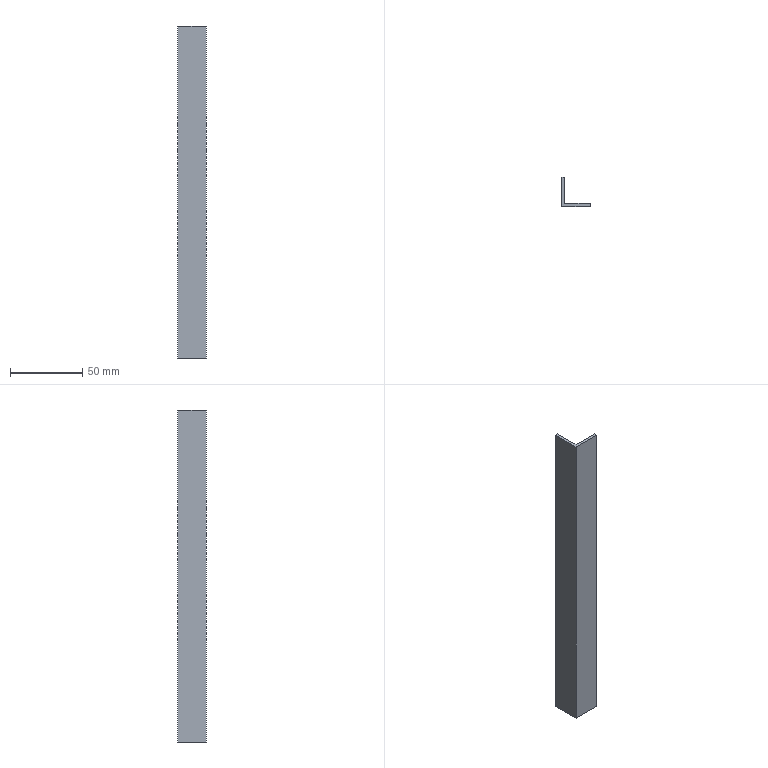Part | STEP file | BCC3 H16_15 | 1 solid | 8 faces | box 20 x 20 x 230 mm | volume 17480 mm3 | plane 8
STEP:
#1=CARTESIAN_POINT('',(0.,0.,0.));
#2=DIRECTION('',(0.,0.,1.));
#3=DIRECTION('',(1.,0.,0.));
#4=AXIS2_PLACEMENT_3D('',#1,#2,#3);
#5=CARTESIAN_POINT('',(0.,0.,-115.));
#6=VERTEX_POINT('',#5);
#7=CARTESIAN_POINT('',(20.,0.,-115.));
#8=VERTEX_POINT('',#7);
#9=CARTESIAN_POINT('',(0.,0.,-115.));
#10=DIRECTION('',(1.,0.,0.));
#11=VECTOR('',#10,1.);
#12=LINE('',#9,#11);
#13=CARTESIAN_POINT('',(0.,0.,115.));
#14=DIRECTION('',(0.,1.,0.));
#15=DIRECTION('',(0.,0.,1.));
#16=AXIS2_PLACEMENT_3D('',#13,#14,#15);
#17=PLANE('',#16);
#18=CARTESIAN_POINT('',(-230.,0.));
#19=DIRECTION('',(0.,1.));
#20=VECTOR('',#19,1.);
#21=LINE('',#18,#20);
#22=(GEOMETRIC_REPRESENTATION_CONTEXT(2)PARAMETRIC_REPRESENTATION_CONTEXT()REPRESENTATION_CONTEXT('',''));
#23=DEFINITIONAL_REPRESENTATION('',(#21),#22);
#24=PCURVE('',#17,#23);
#25=CARTESIAN_POINT('',(0.,0.,-115.));
#26=DIRECTION('',(0.,0.,1.));
#27=DIRECTION('',(1.,0.,0.));
#28=AXIS2_PLACEMENT_3D('',#25,#26,#27);
#29=PLANE('',#28);
#30=CARTESIAN_POINT('',(0.,0.));
#31=DIRECTION('',(1.,0.));
#32=VECTOR('',#31,1.);
#33=LINE('',#30,#32);
#34=(GEOMETRIC_REPRESENTATION_CONTEXT(2)PARAMETRIC_REPRESENTATION_CONTEXT()REPRESENTATION_CONTEXT('',''));
#35=DEFINITIONAL_REPRESENTATION('',(#33),#34);
#36=PCURVE('',#29,#35);
#37=SURFACE_CURVE('',#12,(#24,#36),.PCURVE_S1.);
#38=EDGE_CURVE('',#6,#8,#37,.T.);
#39=ORIENTED_EDGE('',*,*,#38,.T.);
#40=CARTESIAN_POINT('',(20.,0.,115.));
#41=VERTEX_POINT('',#40);
#42=CARTESIAN_POINT('',(20.,0.,115.));
#43=DIRECTION('',(0.,0.,-1.));
#44=VECTOR('',#43,1.);
#45=LINE('',#42,#44);
#46=CARTESIAN_POINT('',(0.,20.));
#47=DIRECTION('',(-1.,0.));
#48=VECTOR('',#47,1.);
#49=LINE('',#46,#48);
#50=(GEOMETRIC_REPRESENTATION_CONTEXT(2)PARAMETRIC_REPRESENTATION_CONTEXT()REPRESENTATION_CONTEXT('',''));
#51=DEFINITIONAL_REPRESENTATION('',(#49),#50);
#52=PCURVE('',#17,#51);
#53=CARTESIAN_POINT('',(20.,0.,115.));
#54=DIRECTION('',(-1.,0.,0.));
#55=DIRECTION('',(0.,0.,1.));
#56=AXIS2_PLACEMENT_3D('',#53,#54,#55);
#57=PLANE('',#56);
#58=CARTESIAN_POINT('',(0.,0.));
#59=DIRECTION('',(-1.,0.));
#60=VECTOR('',#59,1.);
#61=LINE('',#58,#60);
#62=(GEOMETRIC_REPRESENTATION_CONTEXT(2)PARAMETRIC_REPRESENTATION_CONTEXT()REPRESENTATION_CONTEXT('',''));
#63=DEFINITIONAL_REPRESENTATION('',(#61),#62);
#64=PCURVE('',#57,#63);
#65=SURFACE_CURVE('',#45,(#52,#64),.PCURVE_S1.);
#66=EDGE_CURVE('',#41,#8,#65,.T.);
#67=ORIENTED_EDGE('',*,*,#66,.F.);
#68=CARTESIAN_POINT('',(0.,0.,115.));
#69=VERTEX_POINT('',#68);
#70=CARTESIAN_POINT('',(0.,0.,115.));
#71=DIRECTION('',(1.,0.,0.));
#72=VECTOR('',#71,1.);
#73=LINE('',#70,#72);
#74=CARTESIAN_POINT('',(0.,0.));
#75=DIRECTION('',(0.,1.));
#76=VECTOR('',#75,1.);
#77=LINE('',#74,#76);
#78=(GEOMETRIC_REPRESENTATION_CONTEXT(2)PARAMETRIC_REPRESENTATION_CONTEXT()REPRESENTATION_CONTEXT('',''));
#79=DEFINITIONAL_REPRESENTATION('',(#77),#78);
#80=PCURVE('',#17,#79);
#81=CARTESIAN_POINT('',(0.,0.,115.));
#82=DIRECTION('',(0.,0.,1.));
#83=DIRECTION('',(1.,0.,0.));
#84=AXIS2_PLACEMENT_3D('',#81,#82,#83);
#85=PLANE('',#84);
#86=CARTESIAN_POINT('',(0.,0.));
#87=DIRECTION('',(1.,0.));
#88=VECTOR('',#87,1.);
#89=LINE('',#86,#88);
#90=(GEOMETRIC_REPRESENTATION_CONTEXT(2)PARAMETRIC_REPRESENTATION_CONTEXT()REPRESENTATION_CONTEXT('',''));
#91=DEFINITIONAL_REPRESENTATION('',(#89),#90);
#92=PCURVE('',#85,#91);
#93=SURFACE_CURVE('',#73,(#80,#92),.PCURVE_S1.);
#94=EDGE_CURVE('',#69,#41,#93,.T.);
#95=ORIENTED_EDGE('',*,*,#94,.F.);
#96=CARTESIAN_POINT('',(0.,0.,115.));
#97=DIRECTION('',(0.,0.,-1.));
#98=VECTOR('',#97,1.);
#99=LINE('',#96,#98);
#100=CARTESIAN_POINT('',(0.,0.));
#101=DIRECTION('',(-1.,0.));
#102=VECTOR('',#101,1.);
#103=LINE('',#100,#102);
#104=(GEOMETRIC_REPRESENTATION_CONTEXT(2)PARAMETRIC_REPRESENTATION_CONTEXT()REPRESENTATION_CONTEXT('',''));
#105=DEFINITIONAL_REPRESENTATION('',(#103),#104);
#106=PCURVE('',#17,#105);
#107=CARTESIAN_POINT('',(0.,0.,115.));
#108=DIRECTION('',(1.,0.,0.));
#109=DIRECTION('',(0.,0.,-1.));
#110=AXIS2_PLACEMENT_3D('',#107,#108,#109);
#111=PLANE('',#110);
#112=CARTESIAN_POINT('',(0.,0.));
#113=DIRECTION('',(1.,0.));
#114=VECTOR('',#113,1.);
#115=LINE('',#112,#114);
#116=(GEOMETRIC_REPRESENTATION_CONTEXT(2)PARAMETRIC_REPRESENTATION_CONTEXT()REPRESENTATION_CONTEXT('',''));
#117=DEFINITIONAL_REPRESENTATION('',(#115),#116);
#118=PCURVE('',#111,#117);
#119=SURFACE_CURVE('',#99,(#106,#118),.PCURVE_S1.);
#120=EDGE_CURVE('',#69,#6,#119,.T.);
#121=ORIENTED_EDGE('',*,*,#120,.T.);
#122=EDGE_LOOP('',(#39,#67,#95,#121));
#123=FACE_BOUND('',#122,.T.);
#124=ADVANCED_FACE('',(#123),#17,.F.);
#125=CARTESIAN_POINT('',(20.,2.,-115.));
#126=VERTEX_POINT('',#125);
#127=CARTESIAN_POINT('',(20.,0.,-115.));
#128=DIRECTION('',(0.,1.,0.));
#129=VECTOR('',#128,1.);
#130=LINE('',#127,#129);
#131=CARTESIAN_POINT('',(-230.,0.));
#132=DIRECTION('',(0.,1.));
#133=VECTOR('',#132,1.);
#134=LINE('',#131,#133);
#135=(GEOMETRIC_REPRESENTATION_CONTEXT(2)PARAMETRIC_REPRESENTATION_CONTEXT()REPRESENTATION_CONTEXT('',''));
#136=DEFINITIONAL_REPRESENTATION('',(#134),#135);
#137=PCURVE('',#57,#136);
#138=CARTESIAN_POINT('',(20.,0.));
#139=DIRECTION('',(0.,1.));
#140=VECTOR('',#139,1.);
#141=LINE('',#138,#140);
#142=(GEOMETRIC_REPRESENTATION_CONTEXT(2)PARAMETRIC_REPRESENTATION_CONTEXT()REPRESENTATION_CONTEXT('',''));
#143=DEFINITIONAL_REPRESENTATION('',(#141),#142);
#144=PCURVE('',#29,#143);
#145=SURFACE_CURVE('',#130,(#137,#144),.PCURVE_S1.);
#146=EDGE_CURVE('',#8,#126,#145,.T.);
#147=ORIENTED_EDGE('',*,*,#146,.T.);
#148=CARTESIAN_POINT('',(20.,2.,115.));
#149=VERTEX_POINT('',#148);
#150=CARTESIAN_POINT('',(20.,2.,115.));
#151=DIRECTION('',(0.,0.,-1.));
#152=VECTOR('',#151,1.);
#153=LINE('',#150,#152);
#154=CARTESIAN_POINT('',(0.,2.));
#155=DIRECTION('',(-1.,0.));
#156=VECTOR('',#155,1.);
#157=LINE('',#154,#156);
#158=(GEOMETRIC_REPRESENTATION_CONTEXT(2)PARAMETRIC_REPRESENTATION_CONTEXT()REPRESENTATION_CONTEXT('',''));
#159=DEFINITIONAL_REPRESENTATION('',(#157),#158);
#160=PCURVE('',#57,#159);
#161=CARTESIAN_POINT('',(20.,2.,115.));
#162=DIRECTION('',(0.,-1.,0.));
#163=DIRECTION('',(1.,0.,0.));
#164=AXIS2_PLACEMENT_3D('',#161,#162,#163);
#165=PLANE('',#164);
#166=CARTESIAN_POINT('',(0.,0.));
#167=DIRECTION('',(0.,-1.));
#168=VECTOR('',#167,1.);
#169=LINE('',#166,#168);
#170=(GEOMETRIC_REPRESENTATION_CONTEXT(2)PARAMETRIC_REPRESENTATION_CONTEXT()REPRESENTATION_CONTEXT('',''));
#171=DEFINITIONAL_REPRESENTATION('',(#169),#170);
#172=PCURVE('',#165,#171);
#173=SURFACE_CURVE('',#153,(#160,#172),.PCURVE_S1.);
#174=EDGE_CURVE('',#149,#126,#173,.T.);
#175=ORIENTED_EDGE('',*,*,#174,.F.);
#176=CARTESIAN_POINT('',(20.,0.,115.));
#177=DIRECTION('',(0.,1.,0.));
#178=VECTOR('',#177,1.);
#179=LINE('',#176,#178);
#180=CARTESIAN_POINT('',(0.,0.));
#181=DIRECTION('',(0.,1.));
#182=VECTOR('',#181,1.);
#183=LINE('',#180,#182);
#184=(GEOMETRIC_REPRESENTATION_CONTEXT(2)PARAMETRIC_REPRESENTATION_CONTEXT()REPRESENTATION_CONTEXT('',''));
#185=DEFINITIONAL_REPRESENTATION('',(#183),#184);
#186=PCURVE('',#57,#185);
#187=CARTESIAN_POINT('',(20.,0.));
#188=DIRECTION('',(0.,1.));
#189=VECTOR('',#188,1.);
#190=LINE('',#187,#189);
#191=(GEOMETRIC_REPRESENTATION_CONTEXT(2)PARAMETRIC_REPRESENTATION_CONTEXT()REPRESENTATION_CONTEXT('',''));
#192=DEFINITIONAL_REPRESENTATION('',(#190),#191);
#193=PCURVE('',#85,#192);
#194=SURFACE_CURVE('',#179,(#186,#193),.PCURVE_S1.);
#195=EDGE_CURVE('',#41,#149,#194,.T.);
#196=ORIENTED_EDGE('',*,*,#195,.F.);
#197=ORIENTED_EDGE('',*,*,#66,.T.);
#198=EDGE_LOOP('',(#147,#175,#196,#197));
#199=FACE_BOUND('',#198,.T.);
#200=ADVANCED_FACE('',(#199),#57,.F.);
#201=CARTESIAN_POINT('',(2.,2.,-115.));
#202=VERTEX_POINT('',#201);
#203=CARTESIAN_POINT('',(20.,2.,-115.));
#204=DIRECTION('',(-1.,0.,0.));
#205=VECTOR('',#204,1.);
#206=LINE('',#203,#205);
#207=CARTESIAN_POINT('',(0.,-230.));
#208=DIRECTION('',(-1.,0.));
#209=VECTOR('',#208,1.);
#210=LINE('',#207,#209);
#211=(GEOMETRIC_REPRESENTATION_CONTEXT(2)PARAMETRIC_REPRESENTATION_CONTEXT()REPRESENTATION_CONTEXT('',''));
#212=DEFINITIONAL_REPRESENTATION('',(#210),#211);
#213=PCURVE('',#165,#212);
#214=CARTESIAN_POINT('',(20.,2.));
#215=DIRECTION('',(-1.,0.));
#216=VECTOR('',#215,1.);
#217=LINE('',#214,#216);
#218=(GEOMETRIC_REPRESENTATION_CONTEXT(2)PARAMETRIC_REPRESENTATION_CONTEXT()REPRESENTATION_CONTEXT('',''));
#219=DEFINITIONAL_REPRESENTATION('',(#217),#218);
#220=PCURVE('',#29,#219);
#221=SURFACE_CURVE('',#206,(#213,#220),.PCURVE_S1.);
#222=EDGE_CURVE('',#126,#202,#221,.T.);
#223=ORIENTED_EDGE('',*,*,#222,.T.);
#224=CARTESIAN_POINT('',(2.,2.,115.));
#225=VERTEX_POINT('',#224);
#226=CARTESIAN_POINT('',(2.,2.,115.));
#227=DIRECTION('',(0.,0.,-1.));
#228=VECTOR('',#227,1.);
#229=LINE('',#226,#228);
#230=CARTESIAN_POINT('',(-18.,0.));
#231=DIRECTION('',(0.,-1.));
#232=VECTOR('',#231,1.);
#233=LINE('',#230,#232);
#234=(GEOMETRIC_REPRESENTATION_CONTEXT(2)PARAMETRIC_REPRESENTATION_CONTEXT()REPRESENTATION_CONTEXT('',''));
#235=DEFINITIONAL_REPRESENTATION('',(#233),#234);
#236=PCURVE('',#165,#235);
#237=CARTESIAN_POINT('',(2.,2.,115.));
#238=DIRECTION('',(-1.,0.,0.));
#239=DIRECTION('',(0.,-1.,0.));
#240=AXIS2_PLACEMENT_3D('',#237,#238,#239);
#241=PLANE('',#240);
#242=CARTESIAN_POINT('',(0.,0.));
#243=DIRECTION('',(0.,-1.));
#244=VECTOR('',#243,1.);
#245=LINE('',#242,#244);
#246=(GEOMETRIC_REPRESENTATION_CONTEXT(2)PARAMETRIC_REPRESENTATION_CONTEXT()REPRESENTATION_CONTEXT('',''));
#247=DEFINITIONAL_REPRESENTATION('',(#245),#246);
#248=PCURVE('',#241,#247);
#249=SURFACE_CURVE('',#229,(#236,#248),.PCURVE_S1.);
#250=EDGE_CURVE('',#225,#202,#249,.T.);
#251=ORIENTED_EDGE('',*,*,#250,.F.);
#252=CARTESIAN_POINT('',(20.,2.,115.));
#253=DIRECTION('',(-1.,0.,0.));
#254=VECTOR('',#253,1.);
#255=LINE('',#252,#254);
#256=CARTESIAN_POINT('',(0.,0.));
#257=DIRECTION('',(-1.,0.));
#258=VECTOR('',#257,1.);
#259=LINE('',#256,#258);
#260=(GEOMETRIC_REPRESENTATION_CONTEXT(2)PARAMETRIC_REPRESENTATION_CONTEXT()REPRESENTATION_CONTEXT('',''));
#261=DEFINITIONAL_REPRESENTATION('',(#259),#260);
#262=PCURVE('',#165,#261);
#263=CARTESIAN_POINT('',(20.,2.));
#264=DIRECTION('',(-1.,0.));
#265=VECTOR('',#264,1.);
#266=LINE('',#263,#265);
#267=(GEOMETRIC_REPRESENTATION_CONTEXT(2)PARAMETRIC_REPRESENTATION_CONTEXT()REPRESENTATION_CONTEXT('',''));
#268=DEFINITIONAL_REPRESENTATION('',(#266),#267);
#269=PCURVE('',#85,#268);
#270=SURFACE_CURVE('',#255,(#262,#269),.PCURVE_S1.);
#271=EDGE_CURVE('',#149,#225,#270,.T.);
#272=ORIENTED_EDGE('',*,*,#271,.F.);
#273=ORIENTED_EDGE('',*,*,#174,.T.);
#274=EDGE_LOOP('',(#223,#251,#272,#273));
#275=FACE_BOUND('',#274,.T.);
#276=ADVANCED_FACE('',(#275),#165,.F.);
#277=CARTESIAN_POINT('',(2.,20.,-115.));
#278=VERTEX_POINT('',#277);
#279=CARTESIAN_POINT('',(2.,2.,-115.));
#280=DIRECTION('',(0.,1.,0.));
#281=VECTOR('',#280,1.);
#282=LINE('',#279,#281);
#283=CARTESIAN_POINT('',(0.,-230.));
#284=DIRECTION('',(-1.,0.));
#285=VECTOR('',#284,1.);
#286=LINE('',#283,#285);
#287=(GEOMETRIC_REPRESENTATION_CONTEXT(2)PARAMETRIC_REPRESENTATION_CONTEXT()REPRESENTATION_CONTEXT('',''));
#288=DEFINITIONAL_REPRESENTATION('',(#286),#287);
#289=PCURVE('',#241,#288);
#290=CARTESIAN_POINT('',(2.,2.));
#291=DIRECTION('',(0.,1.));
#292=VECTOR('',#291,1.);
#293=LINE('',#290,#292);
#294=(GEOMETRIC_REPRESENTATION_CONTEXT(2)PARAMETRIC_REPRESENTATION_CONTEXT()REPRESENTATION_CONTEXT('',''));
#295=DEFINITIONAL_REPRESENTATION('',(#293),#294);
#296=PCURVE('',#29,#295);
#297=SURFACE_CURVE('',#282,(#289,#296),.PCURVE_S1.);
#298=EDGE_CURVE('',#202,#278,#297,.T.);
#299=ORIENTED_EDGE('',*,*,#298,.T.);
#300=CARTESIAN_POINT('',(2.,20.,115.));
#301=VERTEX_POINT('',#300);
#302=CARTESIAN_POINT('',(2.,20.,115.));
#303=DIRECTION('',(0.,0.,-1.));
#304=VECTOR('',#303,1.);
#305=LINE('',#302,#304);
#306=CARTESIAN_POINT('',(-18.,0.));
#307=DIRECTION('',(0.,-1.));
#308=VECTOR('',#307,1.);
#309=LINE('',#306,#308);
#310=(GEOMETRIC_REPRESENTATION_CONTEXT(2)PARAMETRIC_REPRESENTATION_CONTEXT()REPRESENTATION_CONTEXT('',''));
#311=DEFINITIONAL_REPRESENTATION('',(#309),#310);
#312=PCURVE('',#241,#311);
#313=CARTESIAN_POINT('',(2.,20.,115.));
#314=DIRECTION('',(0.,-1.,0.));
#315=DIRECTION('',(0.,0.,-1.));
#316=AXIS2_PLACEMENT_3D('',#313,#314,#315);
#317=PLANE('',#316);
#318=CARTESIAN_POINT('',(0.,0.));
#319=DIRECTION('',(1.,0.));
#320=VECTOR('',#319,1.);
#321=LINE('',#318,#320);
#322=(GEOMETRIC_REPRESENTATION_CONTEXT(2)PARAMETRIC_REPRESENTATION_CONTEXT()REPRESENTATION_CONTEXT('',''));
#323=DEFINITIONAL_REPRESENTATION('',(#321),#322);
#324=PCURVE('',#317,#323);
#325=SURFACE_CURVE('',#305,(#312,#324),.PCURVE_S1.);
#326=EDGE_CURVE('',#301,#278,#325,.T.);
#327=ORIENTED_EDGE('',*,*,#326,.F.);
#328=CARTESIAN_POINT('',(2.,2.,115.));
#329=DIRECTION('',(0.,1.,0.));
#330=VECTOR('',#329,1.);
#331=LINE('',#328,#330);
#332=CARTESIAN_POINT('',(0.,0.));
#333=DIRECTION('',(-1.,0.));
#334=VECTOR('',#333,1.);
#335=LINE('',#332,#334);
#336=(GEOMETRIC_REPRESENTATION_CONTEXT(2)PARAMETRIC_REPRESENTATION_CONTEXT()REPRESENTATION_CONTEXT('',''));
#337=DEFINITIONAL_REPRESENTATION('',(#335),#336);
#338=PCURVE('',#241,#337);
#339=CARTESIAN_POINT('',(2.,2.));
#340=DIRECTION('',(0.,1.));
#341=VECTOR('',#340,1.);
#342=LINE('',#339,#341);
#343=(GEOMETRIC_REPRESENTATION_CONTEXT(2)PARAMETRIC_REPRESENTATION_CONTEXT()REPRESENTATION_CONTEXT('',''));
#344=DEFINITIONAL_REPRESENTATION('',(#342),#343);
#345=PCURVE('',#85,#344);
#346=SURFACE_CURVE('',#331,(#338,#345),.PCURVE_S1.);
#347=EDGE_CURVE('',#225,#301,#346,.T.);
#348=ORIENTED_EDGE('',*,*,#347,.F.);
#349=ORIENTED_EDGE('',*,*,#250,.T.);
#350=EDGE_LOOP('',(#299,#327,#348,#349));
#351=FACE_BOUND('',#350,.T.);
#352=ADVANCED_FACE('',(#351),#241,.F.);
#353=CARTESIAN_POINT('',(0.,20.,-115.));
#354=VERTEX_POINT('',#353);
#355=CARTESIAN_POINT('',(2.,20.,-115.));
#356=DIRECTION('',(-1.,0.,0.));
#357=VECTOR('',#356,1.);
#358=LINE('',#355,#357);
#359=CARTESIAN_POINT('',(230.,0.));
#360=DIRECTION('',(0.,-1.));
#361=VECTOR('',#360,1.);
#362=LINE('',#359,#361);
#363=(GEOMETRIC_REPRESENTATION_CONTEXT(2)PARAMETRIC_REPRESENTATION_CONTEXT()REPRESENTATION_CONTEXT('',''));
#364=DEFINITIONAL_REPRESENTATION('',(#362),#363);
#365=PCURVE('',#317,#364);
#366=CARTESIAN_POINT('',(2.,20.));
#367=DIRECTION('',(-1.,0.));
#368=VECTOR('',#367,1.);
#369=LINE('',#366,#368);
#370=(GEOMETRIC_REPRESENTATION_CONTEXT(2)PARAMETRIC_REPRESENTATION_CONTEXT()REPRESENTATION_CONTEXT('',''));
#371=DEFINITIONAL_REPRESENTATION('',(#369),#370);
#372=PCURVE('',#29,#371);
#373=SURFACE_CURVE('',#358,(#365,#372),.PCURVE_S1.);
#374=EDGE_CURVE('',#278,#354,#373,.T.);
#375=ORIENTED_EDGE('',*,*,#374,.T.);
#376=CARTESIAN_POINT('',(0.,20.,115.));
#377=VERTEX_POINT('',#376);
#378=CARTESIAN_POINT('',(0.,20.,115.));
#379=DIRECTION('',(0.,0.,-1.));
#380=VECTOR('',#379,1.);
#381=LINE('',#378,#380);
#382=CARTESIAN_POINT('',(0.,-2.));
#383=DIRECTION('',(1.,0.));
#384=VECTOR('',#383,1.);
#385=LINE('',#382,#384);
#386=(GEOMETRIC_REPRESENTATION_CONTEXT(2)PARAMETRIC_REPRESENTATION_CONTEXT()REPRESENTATION_CONTEXT('',''));
#387=DEFINITIONAL_REPRESENTATION('',(#385),#386);
#388=PCURVE('',#317,#387);
#389=CARTESIAN_POINT('',(0.,20.));
#390=DIRECTION('',(1.,0.));
#391=VECTOR('',#390,1.);
#392=LINE('',#389,#391);
#393=(GEOMETRIC_REPRESENTATION_CONTEXT(2)PARAMETRIC_REPRESENTATION_CONTEXT()REPRESENTATION_CONTEXT('',''));
#394=DEFINITIONAL_REPRESENTATION('',(#392),#393);
#395=PCURVE('',#111,#394);
#396=SURFACE_CURVE('',#381,(#388,#395),.PCURVE_S1.);
#397=EDGE_CURVE('',#377,#354,#396,.T.);
#398=ORIENTED_EDGE('',*,*,#397,.F.);
#399=CARTESIAN_POINT('',(2.,20.,115.));
#400=DIRECTION('',(-1.,0.,0.));
#401=VECTOR('',#400,1.);
#402=LINE('',#399,#401);
#403=CARTESIAN_POINT('',(0.,0.));
#404=DIRECTION('',(0.,-1.));
#405=VECTOR('',#404,1.);
#406=LINE('',#403,#405);
#407=(GEOMETRIC_REPRESENTATION_CONTEXT(2)PARAMETRIC_REPRESENTATION_CONTEXT()REPRESENTATION_CONTEXT('',''));
#408=DEFINITIONAL_REPRESENTATION('',(#406),#407);
#409=PCURVE('',#317,#408);
#410=CARTESIAN_POINT('',(2.,20.));
#411=DIRECTION('',(-1.,0.));
#412=VECTOR('',#411,1.);
#413=LINE('',#410,#412);
#414=(GEOMETRIC_REPRESENTATION_CONTEXT(2)PARAMETRIC_REPRESENTATION_CONTEXT()REPRESENTATION_CONTEXT('',''));
#415=DEFINITIONAL_REPRESENTATION('',(#413),#414);
#416=PCURVE('',#85,#415);
#417=SURFACE_CURVE('',#402,(#409,#416),.PCURVE_S1.);
#418=EDGE_CURVE('',#301,#377,#417,.T.);
#419=ORIENTED_EDGE('',*,*,#418,.F.);
#420=ORIENTED_EDGE('',*,*,#326,.T.);
#421=EDGE_LOOP('',(#375,#398,#419,#420));
#422=FACE_BOUND('',#421,.T.);
#423=ADVANCED_FACE('',(#422),#317,.F.);
#424=CARTESIAN_POINT('',(0.,0.,-115.));
#425=DIRECTION('',(0.,-1.,0.));
#426=VECTOR('',#425,1.);
#427=LINE('',#424,#426);
#428=CARTESIAN_POINT('',(230.,0.));
#429=DIRECTION('',(0.,-1.));
#430=VECTOR('',#429,1.);
#431=LINE('',#428,#430);
#432=(GEOMETRIC_REPRESENTATION_CONTEXT(2)PARAMETRIC_REPRESENTATION_CONTEXT()REPRESENTATION_CONTEXT('',''));
#433=DEFINITIONAL_REPRESENTATION('',(#431),#432);
#434=PCURVE('',#111,#433);
#435=CARTESIAN_POINT('',(0.,0.));
#436=DIRECTION('',(0.,-1.));
#437=VECTOR('',#436,1.);
#438=LINE('',#435,#437);
#439=(GEOMETRIC_REPRESENTATION_CONTEXT(2)PARAMETRIC_REPRESENTATION_CONTEXT()REPRESENTATION_CONTEXT('',''));
#440=DEFINITIONAL_REPRESENTATION('',(#438),#439);
#441=PCURVE('',#29,#440);
#442=SURFACE_CURVE('',#427,(#434,#441),.PCURVE_S1.);
#443=EDGE_CURVE('',#354,#6,#442,.T.);
#444=ORIENTED_EDGE('',*,*,#443,.T.);
#445=ORIENTED_EDGE('',*,*,#120,.F.);
#446=CARTESIAN_POINT('',(0.,0.,115.));
#447=DIRECTION('',(0.,-1.,0.));
#448=VECTOR('',#447,1.);
#449=LINE('',#446,#448);
#450=CARTESIAN_POINT('',(0.,0.));
#451=DIRECTION('',(0.,-1.));
#452=VECTOR('',#451,1.);
#453=LINE('',#450,#452);
#454=(GEOMETRIC_REPRESENTATION_CONTEXT(2)PARAMETRIC_REPRESENTATION_CONTEXT()REPRESENTATION_CONTEXT('',''));
#455=DEFINITIONAL_REPRESENTATION('',(#453),#454);
#456=PCURVE('',#111,#455);
#457=CARTESIAN_POINT('',(0.,0.));
#458=DIRECTION('',(0.,-1.));
#459=VECTOR('',#458,1.);
#460=LINE('',#457,#459);
#461=(GEOMETRIC_REPRESENTATION_CONTEXT(2)PARAMETRIC_REPRESENTATION_CONTEXT()REPRESENTATION_CONTEXT('',''));
#462=DEFINITIONAL_REPRESENTATION('',(#460),#461);
#463=PCURVE('',#85,#462);
#464=SURFACE_CURVE('',#449,(#456,#463),.PCURVE_S1.);
#465=EDGE_CURVE('',#377,#69,#464,.T.);
#466=ORIENTED_EDGE('',*,*,#465,.F.);
#467=ORIENTED_EDGE('',*,*,#397,.T.);
#468=EDGE_LOOP('',(#444,#445,#466,#467));
#469=FACE_BOUND('',#468,.T.);
#470=ADVANCED_FACE('',(#469),#111,.F.);
#471=ORIENTED_EDGE('',*,*,#94,.T.);
#472=ORIENTED_EDGE('',*,*,#195,.T.);
#473=ORIENTED_EDGE('',*,*,#271,.T.);
#474=ORIENTED_EDGE('',*,*,#347,.T.);
#475=ORIENTED_EDGE('',*,*,#418,.T.);
#476=ORIENTED_EDGE('',*,*,#465,.T.);
#477=EDGE_LOOP('',(#471,#472,#473,#474,#475,#476));
#478=FACE_BOUND('',#477,.T.);
#479=ADVANCED_FACE('',(#478),#85,.T.);
#480=ORIENTED_EDGE('',*,*,#38,.F.);
#481=ORIENTED_EDGE('',*,*,#443,.F.);
#482=ORIENTED_EDGE('',*,*,#374,.F.);
#483=ORIENTED_EDGE('',*,*,#298,.F.);
#484=ORIENTED_EDGE('',*,*,#222,.F.);
#485=ORIENTED_EDGE('',*,*,#146,.F.);
#486=EDGE_LOOP('',(#480,#481,#482,#483,#484,#485));
#487=FACE_BOUND('',#486,.T.);
#488=ADVANCED_FACE('',(#487),#29,.F.);
#489=CLOSED_SHELL('',(#124,#200,#276,#352,#423,#470,#479,#488));
#490=MANIFOLD_SOLID_BREP('',#489);
#491=(LENGTH_UNIT()NAMED_UNIT(*)SI_UNIT(.MILLI.,.METRE.));
#492=UNCERTAINTY_MEASURE_WITH_UNIT(LENGTH_MEASURE(0.0000001),#491,'','');
#493=(NAMED_UNIT(*)PLANE_ANGLE_UNIT()SI_UNIT($,.RADIAN.));
#494=(NAMED_UNIT(*)SI_UNIT($,.STERADIAN.)SOLID_ANGLE_UNIT());
#495=(GEOMETRIC_REPRESENTATION_CONTEXT(3)GLOBAL_UNCERTAINTY_ASSIGNED_CONTEXT((#492))GLOBAL_UNIT_ASSIGNED_CONTEXT((#491,#493,#494))REPRESENTATION_CONTEXT('',''));
#496=ADVANCED_BREP_SHAPE_REPRESENTATION('',(#4,#490),#495);